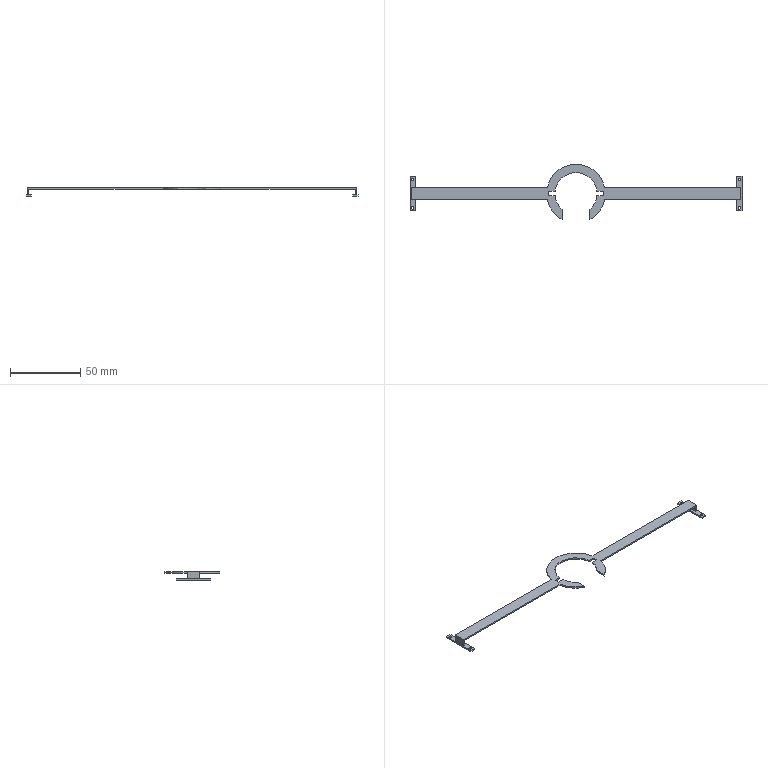Part | SolidWorks | features ICE 2, Extrusion 1 | 1 solid | 44 faces | box 236.176 x 39.297 x 6 mm | volume 2428 mm3 | plane 30 | cylinder 14 | commonest cylinder face diameters 2 x8 30 x3 41.805 x3
STEP:
#1=CARTESIAN_POINT('',(115.275,-10.,-5.));
#2=VERTEX_POINT('',#1);
#3=CARTESIAN_POINT('',(117.275,-10.,-5.));
#4=VERTEX_POINT('',#3);
#5=CARTESIAN_POINT('',(116.275,-10.,-5.));
#6=DIRECTION('',(0.,0.,1.));
#7=DIRECTION('',(-1.,0.,0.));
#8=AXIS2_PLACEMENT_3D('',#5,#6,#7);
#9=CIRCLE('',#8,1.);
#10=EDGE_CURVE('',#2,#4,#9,.T.);
#11=ORIENTED_EDGE('',*,*,#10,.T.);
#12=CARTESIAN_POINT('',(117.275,-10.,-6.));
#13=VERTEX_POINT('',#12);
#14=CARTESIAN_POINT('',(117.275,-10.,-5.));
#15=DIRECTION('',(0.,0.,-1.));
#16=VECTOR('',#15,1000.);
#17=LINE('',#14,#16);
#18=EDGE_CURVE('',#4,#13,#17,.T.);
#19=ORIENTED_EDGE('',*,*,#18,.T.);
#20=CARTESIAN_POINT('',(115.275,-10.,-6.));
#21=VERTEX_POINT('',#20);
#22=CARTESIAN_POINT('',(116.275,-10.,-6.));
#23=DIRECTION('',(0.,0.,1.));
#24=DIRECTION('',(-1.,0.,0.));
#25=AXIS2_PLACEMENT_3D('',#22,#23,#24);
#26=CIRCLE('',#25,1.);
#27=EDGE_CURVE('',#21,#13,#26,.T.);
#28=ORIENTED_EDGE('',*,*,#27,.F.);
#29=CARTESIAN_POINT('',(115.275,-10.,-5.));
#30=DIRECTION('',(0.,0.,-1.));
#31=VECTOR('',#30,1000.);
#32=LINE('',#29,#31);
#33=EDGE_CURVE('',#2,#21,#32,.T.);
#34=ORIENTED_EDGE('',*,*,#33,.F.);
#35=EDGE_LOOP('',(#11,#19,#28,#34));
#36=FACE_OUTER_BOUND('',#35,.T.);
#37=CARTESIAN_POINT('',(116.275,-10.,-5.));
#38=DIRECTION('',(0.,0.,-1.));
#39=DIRECTION('',(-1.,0.,0.));
#40=AXIS2_PLACEMENT_3D('',#37,#38,#39);
#41=CYLINDRICAL_SURFACE('',#40,1.);
#42=ADVANCED_FACE('',(#36),#41,.F.);
#43=CARTESIAN_POINT('',(115.275,10.,-5.));
#44=VERTEX_POINT('',#43);
#45=CARTESIAN_POINT('',(117.275,10.,-5.));
#46=VERTEX_POINT('',#45);
#47=CARTESIAN_POINT('',(116.275,10.,-5.));
#48=DIRECTION('',(0.,0.,1.));
#49=DIRECTION('',(-1.,0.,0.));
#50=AXIS2_PLACEMENT_3D('',#47,#48,#49);
#51=CIRCLE('',#50,1.);
#52=EDGE_CURVE('',#44,#46,#51,.T.);
#53=ORIENTED_EDGE('',*,*,#52,.T.);
#54=CARTESIAN_POINT('',(117.275,10.,-6.));
#55=VERTEX_POINT('',#54);
#56=CARTESIAN_POINT('',(117.275,10.,-5.));
#57=DIRECTION('',(0.,0.,-1.));
#58=VECTOR('',#57,1000.);
#59=LINE('',#56,#58);
#60=EDGE_CURVE('',#46,#55,#59,.T.);
#61=ORIENTED_EDGE('',*,*,#60,.T.);
#62=CARTESIAN_POINT('',(115.275,10.,-6.));
#63=VERTEX_POINT('',#62);
#64=CARTESIAN_POINT('',(116.275,10.,-6.));
#65=DIRECTION('',(0.,0.,1.));
#66=DIRECTION('',(-1.,0.,0.));
#67=AXIS2_PLACEMENT_3D('',#64,#65,#66);
#68=CIRCLE('',#67,1.);
#69=EDGE_CURVE('',#63,#55,#68,.T.);
#70=ORIENTED_EDGE('',*,*,#69,.F.);
#71=CARTESIAN_POINT('',(115.275,10.,-5.));
#72=DIRECTION('',(0.,0.,-1.));
#73=VECTOR('',#72,1000.);
#74=LINE('',#71,#73);
#75=EDGE_CURVE('',#44,#63,#74,.T.);
#76=ORIENTED_EDGE('',*,*,#75,.F.);
#77=EDGE_LOOP('',(#53,#61,#70,#76));
#78=FACE_OUTER_BOUND('',#77,.T.);
#79=CARTESIAN_POINT('',(116.275,10.,-5.));
#80=DIRECTION('',(0.,0.,-1.));
#81=DIRECTION('',(-1.,0.,0.));
#82=AXIS2_PLACEMENT_3D('',#79,#80,#81);
#83=CYLINDRICAL_SURFACE('',#82,1.);
#84=ADVANCED_FACE('',(#78),#83,.F.);
#85=CARTESIAN_POINT('',(-117.275,10.,-5.));
#86=VERTEX_POINT('',#85);
#87=CARTESIAN_POINT('',(-115.275,10.,-5.));
#88=VERTEX_POINT('',#87);
#89=CARTESIAN_POINT('',(-116.275,10.,-5.));
#90=DIRECTION('',(0.,0.,1.));
#91=DIRECTION('',(1.,0.,0.));
#92=AXIS2_PLACEMENT_3D('',#89,#90,#91);
#93=CIRCLE('',#92,1.);
#94=EDGE_CURVE('',#86,#88,#93,.T.);
#95=ORIENTED_EDGE('',*,*,#94,.T.);
#96=CARTESIAN_POINT('',(-115.275,10.,-6.));
#97=VERTEX_POINT('',#96);
#98=CARTESIAN_POINT('',(-115.275,10.,-5.));
#99=DIRECTION('',(0.,0.,-1.));
#100=VECTOR('',#99,1000.);
#101=LINE('',#98,#100);
#102=EDGE_CURVE('',#88,#97,#101,.T.);
#103=ORIENTED_EDGE('',*,*,#102,.T.);
#104=CARTESIAN_POINT('',(-117.275,10.,-6.));
#105=VERTEX_POINT('',#104);
#106=CARTESIAN_POINT('',(-116.275,10.,-6.));
#107=DIRECTION('',(0.,0.,1.));
#108=DIRECTION('',(1.,0.,0.));
#109=AXIS2_PLACEMENT_3D('',#106,#107,#108);
#110=CIRCLE('',#109,1.);
#111=EDGE_CURVE('',#105,#97,#110,.T.);
#112=ORIENTED_EDGE('',*,*,#111,.F.);
#113=CARTESIAN_POINT('',(-117.275,10.,-5.));
#114=DIRECTION('',(0.,0.,-1.));
#115=VECTOR('',#114,1000.);
#116=LINE('',#113,#115);
#117=EDGE_CURVE('',#86,#105,#116,.T.);
#118=ORIENTED_EDGE('',*,*,#117,.F.);
#119=EDGE_LOOP('',(#95,#103,#112,#118));
#120=FACE_OUTER_BOUND('',#119,.T.);
#121=CARTESIAN_POINT('',(-116.275,10.,-5.));
#122=DIRECTION('',(0.,0.,-1.));
#123=DIRECTION('',(-1.,0.,0.));
#124=AXIS2_PLACEMENT_3D('',#121,#122,#123);
#125=CYLINDRICAL_SURFACE('',#124,1.);
#126=ADVANCED_FACE('',(#120),#125,.F.);
#127=CARTESIAN_POINT('',(-117.275,-10.,-5.));
#128=VERTEX_POINT('',#127);
#129=CARTESIAN_POINT('',(-115.275,-10.,-5.));
#130=VERTEX_POINT('',#129);
#131=CARTESIAN_POINT('',(-116.275,-10.,-5.));
#132=DIRECTION('',(0.,0.,1.));
#133=DIRECTION('',(1.,0.,0.));
#134=AXIS2_PLACEMENT_3D('',#131,#132,#133);
#135=CIRCLE('',#134,1.);
#136=EDGE_CURVE('',#128,#130,#135,.T.);
#137=ORIENTED_EDGE('',*,*,#136,.T.);
#138=CARTESIAN_POINT('',(-115.275,-10.,-6.));
#139=VERTEX_POINT('',#138);
#140=CARTESIAN_POINT('',(-115.275,-10.,-5.));
#141=DIRECTION('',(0.,0.,-1.));
#142=VECTOR('',#141,1000.);
#143=LINE('',#140,#142);
#144=EDGE_CURVE('',#130,#139,#143,.T.);
#145=ORIENTED_EDGE('',*,*,#144,.T.);
#146=CARTESIAN_POINT('',(-117.275,-10.,-6.));
#147=VERTEX_POINT('',#146);
#148=CARTESIAN_POINT('',(-116.275,-10.,-6.));
#149=DIRECTION('',(0.,0.,1.));
#150=DIRECTION('',(1.,0.,0.));
#151=AXIS2_PLACEMENT_3D('',#148,#149,#150);
#152=CIRCLE('',#151,1.);
#153=EDGE_CURVE('',#147,#139,#152,.T.);
#154=ORIENTED_EDGE('',*,*,#153,.F.);
#155=CARTESIAN_POINT('',(-117.275,-10.,-5.));
#156=DIRECTION('',(0.,0.,-1.));
#157=VECTOR('',#156,1000.);
#158=LINE('',#155,#157);
#159=EDGE_CURVE('',#128,#147,#158,.T.);
#160=ORIENTED_EDGE('',*,*,#159,.F.);
#161=EDGE_LOOP('',(#137,#145,#154,#160));
#162=FACE_OUTER_BOUND('',#161,.T.);
#163=CARTESIAN_POINT('',(-116.275,-10.,-5.));
#164=DIRECTION('',(0.,0.,-1.));
#165=DIRECTION('',(-1.,0.,0.));
#166=AXIS2_PLACEMENT_3D('',#163,#164,#165);
#167=CYLINDRICAL_SURFACE('',#166,1.);
#168=ADVANCED_FACE('',(#162),#167,.F.);
#169=CARTESIAN_POINT('',(116.275,-4.349,-5.));
#170=VERTEX_POINT('',#169);
#171=CARTESIAN_POINT('',(116.275,-4.349,-1.));
#172=VERTEX_POINT('',#171);
#173=CARTESIAN_POINT('',(116.275,-4.349,-14.755));
#174=DIRECTION('',(0.,0.,1.));
#175=VECTOR('',#174,1000.);
#176=LINE('',#173,#175);
#177=EDGE_CURVE('',#170,#172,#176,.T.);
#178=ORIENTED_EDGE('',*,*,#177,.F.);
#179=CARTESIAN_POINT('',(117.275,-4.349,-5.));
#180=VERTEX_POINT('',#179);
#181=CARTESIAN_POINT('',(20.445,-4.349,-5.));
#182=DIRECTION('',(1.,0.,0.));
#183=VECTOR('',#182,1000.);
#184=LINE('',#181,#183);
#185=EDGE_CURVE('',#170,#180,#184,.T.);
#186=ORIENTED_EDGE('',*,*,#185,.T.);
#187=CARTESIAN_POINT('',(117.275,-4.349,0.));
#188=VERTEX_POINT('',#187);
#189=CARTESIAN_POINT('',(117.275,-4.349,-1.));
#190=DIRECTION('',(0.,0.,1.));
#191=VECTOR('',#190,1000.);
#192=LINE('',#189,#191);
#193=EDGE_CURVE('',#180,#188,#192,.T.);
#194=ORIENTED_EDGE('',*,*,#193,.T.);
#195=CARTESIAN_POINT('',(20.445,-4.349,0.));
#196=VERTEX_POINT('',#195);
#197=CARTESIAN_POINT('',(20.445,-4.349,0.));
#198=DIRECTION('',(1.,0.,0.));
#199=VECTOR('',#198,1000.);
#200=LINE('',#197,#199);
#201=EDGE_CURVE('',#196,#188,#200,.T.);
#202=ORIENTED_EDGE('',*,*,#201,.F.);
#203=CARTESIAN_POINT('',(20.445,-4.349,-1.));
#204=VERTEX_POINT('',#203);
#205=CARTESIAN_POINT('',(20.445,-4.349,-1.));
#206=DIRECTION('',(0.,0.,1.));
#207=VECTOR('',#206,1000.);
#208=LINE('',#205,#207);
#209=EDGE_CURVE('',#204,#196,#208,.T.);
#210=ORIENTED_EDGE('',*,*,#209,.F.);
#211=CARTESIAN_POINT('',(20.445,-4.349,-1.));
#212=DIRECTION('',(1.,0.,0.));
#213=VECTOR('',#212,1000.);
#214=LINE('',#211,#213);
#215=EDGE_CURVE('',#204,#172,#214,.T.);
#216=ORIENTED_EDGE('',*,*,#215,.T.);
#217=EDGE_LOOP('',(#178,#186,#194,#202,#210,#216));
#218=FACE_OUTER_BOUND('',#217,.T.);
#219=CARTESIAN_POINT('',(20.445,-4.349,-1.));
#220=DIRECTION('',(0.,-1.,0.));
#221=DIRECTION('',(0.,0.,-1.));
#222=AXIS2_PLACEMENT_3D('',#219,#220,#221);
#223=PLANE('',#222);
#224=ADVANCED_FACE('',(#218),#223,.T.);
#225=CARTESIAN_POINT('',(117.275,4.349,-5.));
#226=VERTEX_POINT('',#225);
#227=CARTESIAN_POINT('',(117.275,4.349,0.));
#228=VERTEX_POINT('',#227);
#229=CARTESIAN_POINT('',(117.275,4.349,-1.));
#230=DIRECTION('',(0.,0.,1.));
#231=VECTOR('',#230,1000.);
#232=LINE('',#229,#231);
#233=EDGE_CURVE('',#226,#228,#232,.T.);
#234=ORIENTED_EDGE('',*,*,#233,.F.);
#235=CARTESIAN_POINT('',(116.275,4.349,-5.));
#236=VERTEX_POINT('',#235);
#237=CARTESIAN_POINT('',(20.445,4.349,-5.));
#238=DIRECTION('',(-1.,0.,0.));
#239=VECTOR('',#238,1000.);
#240=LINE('',#237,#239);
#241=EDGE_CURVE('',#226,#236,#240,.T.);
#242=ORIENTED_EDGE('',*,*,#241,.T.);
#243=CARTESIAN_POINT('',(116.275,4.349,-1.));
#244=VERTEX_POINT('',#243);
#245=CARTESIAN_POINT('',(116.275,4.349,-14.755));
#246=DIRECTION('',(0.,0.,1.));
#247=VECTOR('',#246,1000.);
#248=LINE('',#245,#247);
#249=EDGE_CURVE('',#236,#244,#248,.T.);
#250=ORIENTED_EDGE('',*,*,#249,.T.);
#251=CARTESIAN_POINT('',(20.445,4.349,-1.));
#252=VERTEX_POINT('',#251);
#253=CARTESIAN_POINT('',(20.445,4.349,-1.));
#254=DIRECTION('',(-1.,0.,0.));
#255=VECTOR('',#254,1000.);
#256=LINE('',#253,#255);
#257=EDGE_CURVE('',#244,#252,#256,.T.);
#258=ORIENTED_EDGE('',*,*,#257,.T.);
#259=CARTESIAN_POINT('',(20.445,4.349,0.));
#260=VERTEX_POINT('',#259);
#261=CARTESIAN_POINT('',(20.445,4.349,-1.));
#262=DIRECTION('',(0.,0.,1.));
#263=VECTOR('',#262,1000.);
#264=LINE('',#261,#263);
#265=EDGE_CURVE('',#252,#260,#264,.T.);
#266=ORIENTED_EDGE('',*,*,#265,.T.);
#267=CARTESIAN_POINT('',(20.445,4.349,0.));
#268=DIRECTION('',(-1.,0.,0.));
#269=VECTOR('',#268,1000.);
#270=LINE('',#267,#269);
#271=EDGE_CURVE('',#228,#260,#270,.T.);
#272=ORIENTED_EDGE('',*,*,#271,.F.);
#273=EDGE_LOOP('',(#234,#242,#250,#258,#266,#272));
#274=FACE_OUTER_BOUND('',#273,.T.);
#275=CARTESIAN_POINT('',(20.445,4.349,-1.));
#276=DIRECTION('',(0.,1.,0.));
#277=DIRECTION('',(0.,0.,1.));
#278=AXIS2_PLACEMENT_3D('',#275,#276,#277);
#279=PLANE('',#278);
#280=ADVANCED_FACE('',(#274),#279,.T.);
#281=ORIENTED_EDGE('',*,*,#193,.F.);
#282=CARTESIAN_POINT('',(117.275,4.349,-5.));
#283=DIRECTION('',(0.,1.,0.));
#284=VECTOR('',#283,1000.);
#285=LINE('',#282,#284);
#286=EDGE_CURVE('',#180,#226,#285,.T.);
#287=ORIENTED_EDGE('',*,*,#286,.T.);
#288=ORIENTED_EDGE('',*,*,#233,.T.);
#289=CARTESIAN_POINT('',(117.275,4.349,0.));
#290=DIRECTION('',(0.,1.,0.));
#291=VECTOR('',#290,1000.);
#292=LINE('',#289,#291);
#293=EDGE_CURVE('',#188,#228,#292,.T.);
#294=ORIENTED_EDGE('',*,*,#293,.F.);
#295=EDGE_LOOP('',(#281,#287,#288,#294));
#296=FACE_OUTER_BOUND('',#295,.T.);
#297=CARTESIAN_POINT('',(117.275,4.349,-1.));
#298=DIRECTION('',(1.,0.,0.));
#299=DIRECTION('',(0.,0.,-1.));
#300=AXIS2_PLACEMENT_3D('',#297,#298,#299);
#301=PLANE('',#300);
#302=ADVANCED_FACE('',(#296),#301,.T.);
#303=ORIENTED_EDGE('',*,*,#249,.F.);
#304=CARTESIAN_POINT('',(116.275,4.349,-5.));
#305=DIRECTION('',(0.,-1.,0.));
#306=VECTOR('',#305,1000.);
#307=LINE('',#304,#306);
#308=EDGE_CURVE('',#236,#170,#307,.T.);
#309=ORIENTED_EDGE('',*,*,#308,.T.);
#310=ORIENTED_EDGE('',*,*,#177,.T.);
#311=CARTESIAN_POINT('',(116.275,0.,-1.));
#312=DIRECTION('',(0.,-1.,0.));
#313=VECTOR('',#312,1000.);
#314=LINE('',#311,#313);
#315=EDGE_CURVE('',#244,#172,#314,.T.);
#316=ORIENTED_EDGE('',*,*,#315,.F.);
#317=EDGE_LOOP('',(#303,#309,#310,#316));
#318=FACE_OUTER_BOUND('',#317,.T.);
#319=CARTESIAN_POINT('',(116.275,4.349,-14.755));
#320=DIRECTION('',(-1.,0.,0.));
#321=DIRECTION('',(0.,0.,1.));
#322=AXIS2_PLACEMENT_3D('',#319,#320,#321);
#323=PLANE('',#322);
#324=ADVANCED_FACE('',(#318),#323,.T.);
#325=CARTESIAN_POINT('',(9.927,-18.395,0.));
#326=VERTEX_POINT('',#325);
#327=CARTESIAN_POINT('',(0.,0.,0.));
#328=DIRECTION('',(0.,0.,1.));
#329=DIRECTION('',(1.,0.,0.));
#330=AXIS2_PLACEMENT_3D('',#327,#328,#329);
#331=CIRCLE('',#330,20.903);
#332=EDGE_CURVE('',#326,#196,#331,.T.);
#333=ORIENTED_EDGE('',*,*,#332,.F.);
#334=CARTESIAN_POINT('',(9.927,-18.395,-1.));
#335=VERTEX_POINT('',#334);
#336=CARTESIAN_POINT('',(9.927,-18.395,-1.));
#337=DIRECTION('',(0.,0.,1.));
#338=VECTOR('',#337,1000.);
#339=LINE('',#336,#338);
#340=EDGE_CURVE('',#335,#326,#339,.T.);
#341=ORIENTED_EDGE('',*,*,#340,.F.);
#342=CARTESIAN_POINT('',(0.,0.,-1.));
#343=DIRECTION('',(0.,0.,1.));
#344=DIRECTION('',(1.,0.,0.));
#345=AXIS2_PLACEMENT_3D('',#342,#343,#344);
#346=CIRCLE('',#345,20.903);
#347=EDGE_CURVE('',#335,#204,#346,.T.);
#348=ORIENTED_EDGE('',*,*,#347,.T.);
#349=ORIENTED_EDGE('',*,*,#209,.T.);
#350=EDGE_LOOP('',(#333,#341,#348,#349));
#351=FACE_OUTER_BOUND('',#350,.T.);
#352=CARTESIAN_POINT('',(0.,0.,-1.));
#353=DIRECTION('',(0.,0.,1.));
#354=DIRECTION('',(1.,0.,0.));
#355=AXIS2_PLACEMENT_3D('',#352,#353,#354);
#356=CYLINDRICAL_SURFACE('',#355,20.903);
#357=ADVANCED_FACE('',(#351),#356,.T.);
#358=CARTESIAN_POINT('',(9.927,-11.245,0.));
#359=VERTEX_POINT('',#358);
#360=CARTESIAN_POINT('',(9.927,-11.245,0.));
#361=DIRECTION('',(0.,-1.,0.));
#362=VECTOR('',#361,1000.);
#363=LINE('',#360,#362);
#364=EDGE_CURVE('',#359,#326,#363,.T.);
#365=ORIENTED_EDGE('',*,*,#364,.F.);
#366=CARTESIAN_POINT('',(9.927,-11.245,-1.));
#367=VERTEX_POINT('',#366);
#368=CARTESIAN_POINT('',(9.927,-11.245,-1.));
#369=DIRECTION('',(0.,0.,1.));
#370=VECTOR('',#369,1000.);
#371=LINE('',#368,#370);
#372=EDGE_CURVE('',#367,#359,#371,.T.);
#373=ORIENTED_EDGE('',*,*,#372,.F.);
#374=CARTESIAN_POINT('',(9.927,-11.245,-1.));
#375=DIRECTION('',(0.,-1.,0.));
#376=VECTOR('',#375,1000.);
#377=LINE('',#374,#376);
#378=EDGE_CURVE('',#367,#335,#377,.T.);
#379=ORIENTED_EDGE('',*,*,#378,.T.);
#380=ORIENTED_EDGE('',*,*,#340,.T.);
#381=EDGE_LOOP('',(#365,#373,#379,#380));
#382=FACE_OUTER_BOUND('',#381,.T.);
#383=CARTESIAN_POINT('',(9.927,-11.245,-1.));
#384=DIRECTION('',(-1.,0.,0.));
#385=DIRECTION('',(0.,0.,1.));
#386=AXIS2_PLACEMENT_3D('',#383,#384,#385);
#387=PLANE('',#386);
#388=ADVANCED_FACE('',(#382),#387,.T.);
#389=CARTESIAN_POINT('',(14.91,-1.641,0.));
#390=VERTEX_POINT('',#389);
#391=CARTESIAN_POINT('',(0.,0.,0.));
#392=DIRECTION('',(0.,0.,-1.));
#393=DIRECTION('',(1.,0.,0.));
#394=AXIS2_PLACEMENT_3D('',#391,#392,#393);
#395=CIRCLE('',#394,15.);
#396=EDGE_CURVE('',#390,#359,#395,.T.);
#397=ORIENTED_EDGE('',*,*,#396,.F.);
#398=CARTESIAN_POINT('',(14.91,-1.641,-1.));
#399=VERTEX_POINT('',#398);
#400=CARTESIAN_POINT('',(14.91,-1.641,-1.));
#401=DIRECTION('',(0.,0.,1.));
#402=VECTOR('',#401,1000.);
#403=LINE('',#400,#402);
#404=EDGE_CURVE('',#399,#390,#403,.T.);
#405=ORIENTED_EDGE('',*,*,#404,.F.);
#406=CARTESIAN_POINT('',(0.,0.,-1.));
#407=DIRECTION('',(0.,0.,-1.));
#408=DIRECTION('',(1.,0.,0.));
#409=AXIS2_PLACEMENT_3D('',#406,#407,#408);
#410=CIRCLE('',#409,15.);
#411=EDGE_CURVE('',#399,#367,#410,.T.);
#412=ORIENTED_EDGE('',*,*,#411,.T.);
#413=ORIENTED_EDGE('',*,*,#372,.T.);
#414=EDGE_LOOP('',(#397,#405,#412,#413));
#415=FACE_OUTER_BOUND('',#414,.T.);
#416=CARTESIAN_POINT('',(0.,0.,-1.));
#417=DIRECTION('',(0.,0.,1.));
#418=DIRECTION('',(1.,0.,0.));
#419=AXIS2_PLACEMENT_3D('',#416,#417,#418);
#420=CYLINDRICAL_SURFACE('',#419,15.);
#421=ADVANCED_FACE('',(#415),#420,.F.);
#422=CARTESIAN_POINT('',(19.244,-1.641,0.));
#423=VERTEX_POINT('',#422);
#424=CARTESIAN_POINT('',(14.91,-1.641,0.));
#425=DIRECTION('',(-1.,0.,0.));
#426=VECTOR('',#425,1000.);
#427=LINE('',#424,#426);
#428=EDGE_CURVE('',#423,#390,#427,.T.);
#429=ORIENTED_EDGE('',*,*,#428,.F.);
#430=CARTESIAN_POINT('',(19.244,-1.641,-1.));
#431=VERTEX_POINT('',#430);
#432=CARTESIAN_POINT('',(19.244,-1.641,-1.));
#433=DIRECTION('',(0.,0.,1.));
#434=VECTOR('',#433,1000.);
#435=LINE('',#432,#434);
#436=EDGE_CURVE('',#431,#423,#435,.T.);
#437=ORIENTED_EDGE('',*,*,#436,.F.);
#438=CARTESIAN_POINT('',(14.91,-1.641,-1.));
#439=DIRECTION('',(-1.,0.,0.));
#440=VECTOR('',#439,1000.);
#441=LINE('',#438,#440);
#442=EDGE_CURVE('',#431,#399,#441,.T.);
#443=ORIENTED_EDGE('',*,*,#442,.T.);
#444=ORIENTED_EDGE('',*,*,#404,.T.);
#445=EDGE_LOOP('',(#429,#437,#443,#444));
#446=FACE_OUTER_BOUND('',#445,.T.);
#447=CARTESIAN_POINT('',(14.91,-1.641,-1.));
#448=DIRECTION('',(0.,1.,0.));
#449=DIRECTION('',(0.,0.,1.));
#450=AXIS2_PLACEMENT_3D('',#447,#448,#449);
#451=PLANE('',#450);
#452=ADVANCED_FACE('',(#446),#451,.T.);
#453=CARTESIAN_POINT('',(19.244,1.641,0.));
#454=VERTEX_POINT('',#453);
#455=CARTESIAN_POINT('',(19.244,-1.641,0.));
#456=DIRECTION('',(0.,-1.,0.));
#457=VECTOR('',#456,1000.);
#458=LINE('',#455,#457);
#459=EDGE_CURVE('',#454,#423,#458,.T.);
#460=ORIENTED_EDGE('',*,*,#459,.F.);
#461=CARTESIAN_POINT('',(19.244,1.641,-1.));
#462=VERTEX_POINT('',#461);
#463=CARTESIAN_POINT('',(19.244,1.641,-1.));
#464=DIRECTION('',(0.,0.,1.));
#465=VECTOR('',#464,1000.);
#466=LINE('',#463,#465);
#467=EDGE_CURVE('',#462,#454,#466,.T.);
#468=ORIENTED_EDGE('',*,*,#467,.F.);
#469=CARTESIAN_POINT('',(19.244,-1.641,-1.));
#470=DIRECTION('',(0.,-1.,0.));
#471=VECTOR('',#470,1000.);
#472=LINE('',#469,#471);
#473=EDGE_CURVE('',#462,#431,#472,.T.);
#474=ORIENTED_EDGE('',*,*,#473,.T.);
#475=ORIENTED_EDGE('',*,*,#436,.T.);
#476=EDGE_LOOP('',(#460,#468,#474,#475));
#477=FACE_OUTER_BOUND('',#476,.T.);
#478=CARTESIAN_POINT('',(19.244,-1.641,-1.));
#479=DIRECTION('',(-1.,0.,0.));
#480=DIRECTION('',(0.,0.,1.));
#481=AXIS2_PLACEMENT_3D('',#478,#479,#480);
#482=PLANE('',#481);
#483=ADVANCED_FACE('',(#477),#482,.T.);
#484=CARTESIAN_POINT('',(14.91,1.641,0.));
#485=VERTEX_POINT('',#484);
#486=CARTESIAN_POINT('',(14.91,1.641,0.));
#487=DIRECTION('',(1.,0.,0.));
#488=VECTOR('',#487,1000.);
#489=LINE('',#486,#488);
#490=EDGE_CURVE('',#485,#454,#489,.T.);
#491=ORIENTED_EDGE('',*,*,#490,.F.);
#492=CARTESIAN_POINT('',(14.91,1.641,-1.));
#493=VERTEX_POINT('',#492);
#494=CARTESIAN_POINT('',(14.91,1.641,-1.));
#495=DIRECTION('',(0.,0.,1.));
#496=VECTOR('',#495,1000.);
#497=LINE('',#494,#496);
#498=EDGE_CURVE('',#493,#485,#497,.T.);
#499=ORIENTED_EDGE('',*,*,#498,.F.);
#500=CARTESIAN_POINT('',(14.91,1.641,-1.));
#501=DIRECTION('',(1.,0.,0.));
#502=VECTOR('',#501,1000.);
#503=LINE('',#500,#502);
#504=EDGE_CURVE('',#493,#462,#503,.T.);
#505=ORIENTED_EDGE('',*,*,#504,.T.);
#506=ORIENTED_EDGE('',*,*,#467,.T.);
#507=EDGE_LOOP('',(#491,#499,#505,#506));
#508=FACE_OUTER_BOUND('',#507,.T.);
#509=CARTESIAN_POINT('',(14.91,1.641,-1.));
#510=DIRECTION('',(0.,-1.,0.));
#511=DIRECTION('',(0.,0.,-1.));
#512=AXIS2_PLACEMENT_3D('',#509,#510,#511);
#513=PLANE('',#512);
#514=ADVANCED_FACE('',(#508),#513,.T.);
#515=CARTESIAN_POINT('',(-14.91,1.641,0.));
#516=VERTEX_POINT('',#515);
#517=CARTESIAN_POINT('',(0.,0.,0.));
#518=DIRECTION('',(0.,0.,-1.));
#519=DIRECTION('',(1.,0.,0.));
#520=AXIS2_PLACEMENT_3D('',#517,#518,#519);
#521=CIRCLE('',#520,15.);
#522=EDGE_CURVE('',#516,#485,#521,.T.);
#523=ORIENTED_EDGE('',*,*,#522,.F.);
#524=CARTESIAN_POINT('',(-14.91,1.641,-1.));
#525=VERTEX_POINT('',#524);
#526=CARTESIAN_POINT('',(-14.91,1.641,-1.));
#527=DIRECTION('',(0.,0.,1.));
#528=VECTOR('',#527,1000.);
#529=LINE('',#526,#528);
#530=EDGE_CURVE('',#525,#516,#529,.T.);
#531=ORIENTED_EDGE('',*,*,#530,.F.);
#532=CARTESIAN_POINT('',(0.,0.,-1.));
#533=DIRECTION('',(0.,0.,-1.));
#534=DIRECTION('',(1.,0.,0.));
#535=AXIS2_PLACEMENT_3D('',#532,#533,#534);
#536=CIRCLE('',#535,15.);
#537=EDGE_CURVE('',#525,#493,#536,.T.);
#538=ORIENTED_EDGE('',*,*,#537,.T.);
#539=ORIENTED_EDGE('',*,*,#498,.T.);
#540=EDGE_LOOP('',(#523,#531,#538,#539));
#541=FACE_OUTER_BOUND('',#540,.T.);
#542=CARTESIAN_POINT('',(0.,0.,-1.));
#543=DIRECTION('',(0.,0.,1.));
#544=DIRECTION('',(1.,0.,0.));
#545=AXIS2_PLACEMENT_3D('',#542,#543,#544);
#546=CYLINDRICAL_SURFACE('',#545,15.);
#547=ADVANCED_FACE('',(#541),#546,.F.);
#548=CARTESIAN_POINT('',(-19.244,1.641,0.));
#549=VERTEX_POINT('',#548);
#550=CARTESIAN_POINT('',(-19.244,1.641,0.));
#551=DIRECTION('',(1.,0.,0.));
#552=VECTOR('',#551,1000.);
#553=LINE('',#550,#552);
#554=EDGE_CURVE('',#549,#516,#553,.T.);
#555=ORIENTED_EDGE('',*,*,#554,.F.);
#556=CARTESIAN_POINT('',(-19.244,1.641,-1.));
#557=VERTEX_POINT('',#556);
#558=CARTESIAN_POINT('',(-19.244,1.641,-1.));
#559=DIRECTION('',(0.,0.,1.));
#560=VECTOR('',#559,1000.);
#561=LINE('',#558,#560);
#562=EDGE_CURVE('',#557,#549,#561,.T.);
#563=ORIENTED_EDGE('',*,*,#562,.F.);
#564=CARTESIAN_POINT('',(-19.244,1.641,-1.));
#565=DIRECTION('',(1.,0.,0.));
#566=VECTOR('',#565,1000.);
#567=LINE('',#564,#566);
#568=EDGE_CURVE('',#557,#525,#567,.T.);
#569=ORIENTED_EDGE('',*,*,#568,.T.);
#570=ORIENTED_EDGE('',*,*,#530,.T.);
#571=EDGE_LOOP('',(#555,#563,#569,#570));
#572=FACE_OUTER_BOUND('',#571,.T.);
#573=CARTESIAN_POINT('',(-19.244,1.641,-1.));
#574=DIRECTION('',(0.,-1.,0.));
#575=DIRECTION('',(0.,0.,-1.));
#576=AXIS2_PLACEMENT_3D('',#573,#574,#575);
#577=PLANE('',#576);
#578=ADVANCED_FACE('',(#572),#577,.T.);
#579=CARTESIAN_POINT('',(-19.244,-1.641,0.));
#580=VERTEX_POINT('',#579);
#581=CARTESIAN_POINT('',(-19.244,-1.641,0.));
#582=DIRECTION('',(0.,1.,0.));
#583=VECTOR('',#582,1000.);
#584=LINE('',#581,#583);
#585=EDGE_CURVE('',#580,#549,#584,.T.);
#586=ORIENTED_EDGE('',*,*,#585,.F.);
#587=CARTESIAN_POINT('',(-19.244,-1.641,-1.));
#588=VERTEX_POINT('',#587);
#589=CARTESIAN_POINT('',(-19.244,-1.641,-1.));
#590=DIRECTION('',(0.,0.,1.));
#591=VECTOR('',#590,1000.);
#592=LINE('',#589,#591);
#593=EDGE_CURVE('',#588,#580,#592,.T.);
#594=ORIENTED_EDGE('',*,*,#593,.F.);
#595=CARTESIAN_POINT('',(-19.244,-1.641,-1.));
#596=DIRECTION('',(0.,1.,0.));
#597=VECTOR('',#596,1000.);
#598=LINE('',#595,#597);
#599=EDGE_CURVE('',#588,#557,#598,.T.);
#600=ORIENTED_EDGE('',*,*,#599,.T.);
#601=ORIENTED_EDGE('',*,*,#562,.T.);
#602=EDGE_LOOP('',(#586,#594,#600,#601));
#603=FACE_OUTER_BOUND('',#602,.T.);
#604=CARTESIAN_POINT('',(-19.244,-1.641,-1.));
#605=DIRECTION('',(1.,0.,0.));
#606=DIRECTION('',(0.,0.,-1.));
#607=AXIS2_PLACEMENT_3D('',#604,#605,#606);
#608=PLANE('',#607);
#609=ADVANCED_FACE('',(#603),#608,.T.);
#610=CARTESIAN_POINT('',(-14.91,-1.641,0.));
#611=VERTEX_POINT('',#610);
#612=CARTESIAN_POINT('',(-19.244,-1.641,0.));
#613=DIRECTION('',(-1.,0.,0.));
#614=VECTOR('',#613,1000.);
#615=LINE('',#612,#614);
#616=EDGE_CURVE('',#611,#580,#615,.T.);
#617=ORIENTED_EDGE('',*,*,#616,.F.);
#618=CARTESIAN_POINT('',(-14.91,-1.641,-1.));
#619=VERTEX_POINT('',#618);
#620=CARTESIAN_POINT('',(-14.91,-1.641,-1.));
#621=DIRECTION('',(0.,0.,1.));
#622=VECTOR('',#621,1000.);
#623=LINE('',#620,#622);
#624=EDGE_CURVE('',#619,#611,#623,.T.);
#625=ORIENTED_EDGE('',*,*,#624,.F.);
#626=CARTESIAN_POINT('',(-19.244,-1.641,-1.));
#627=DIRECTION('',(-1.,0.,0.));
#628=VECTOR('',#627,1000.);
#629=LINE('',#626,#628);
#630=EDGE_CURVE('',#619,#588,#629,.T.);
#631=ORIENTED_EDGE('',*,*,#630,.T.);
#632=ORIENTED_EDGE('',*,*,#593,.T.);
#633=EDGE_LOOP('',(#617,#625,#631,#632));
#634=FACE_OUTER_BOUND('',#633,.T.);
#635=CARTESIAN_POINT('',(-19.244,-1.641,-1.));
#636=DIRECTION('',(0.,1.,0.));
#637=DIRECTION('',(0.,0.,1.));
#638=AXIS2_PLACEMENT_3D('',#635,#636,#637);
#639=PLANE('',#638);
#640=ADVANCED_FACE('',(#634),#639,.T.);
#641=CARTESIAN_POINT('',(-9.927,-11.245,0.));
#642=VERTEX_POINT('',#641);
#643=CARTESIAN_POINT('',(0.,0.,0.));
#644=DIRECTION('',(0.,0.,-1.));
#645=DIRECTION('',(1.,0.,0.));
#646=AXIS2_PLACEMENT_3D('',#643,#644,#645);
#647=CIRCLE('',#646,15.);
#648=EDGE_CURVE('',#642,#611,#647,.T.);
#649=ORIENTED_EDGE('',*,*,#648,.F.);
#650=CARTESIAN_POINT('',(-9.927,-11.245,-1.));
#651=VERTEX_POINT('',#650);
#652=CARTESIAN_POINT('',(-9.927,-11.245,-1.));
#653=DIRECTION('',(0.,0.,1.));
#654=VECTOR('',#653,1000.);
#655=LINE('',#652,#654);
#656=EDGE_CURVE('',#651,#642,#655,.T.);
#657=ORIENTED_EDGE('',*,*,#656,.F.);
#658=CARTESIAN_POINT('',(0.,0.,-1.));
#659=DIRECTION('',(0.,0.,-1.));
#660=DIRECTION('',(1.,0.,0.));
#661=AXIS2_PLACEMENT_3D('',#658,#659,#660);
#662=CIRCLE('',#661,15.);
#663=EDGE_CURVE('',#651,#619,#662,.T.);
#664=ORIENTED_EDGE('',*,*,#663,.T.);
#665=ORIENTED_EDGE('',*,*,#624,.T.);
#666=EDGE_LOOP('',(#649,#657,#664,#665));
#667=FACE_OUTER_BOUND('',#666,.T.);
#668=CARTESIAN_POINT('',(0.,0.,-1.));
#669=DIRECTION('',(0.,0.,1.));
#670=DIRECTION('',(1.,0.,0.));
#671=AXIS2_PLACEMENT_3D('',#668,#669,#670);
#672=CYLINDRICAL_SURFACE('',#671,15.);
#673=ADVANCED_FACE('',(#667),#672,.F.);
#674=CARTESIAN_POINT('',(-9.927,-18.395,0.));
#675=VERTEX_POINT('',#674);
#676=CARTESIAN_POINT('',(-9.927,-11.245,0.));
#677=DIRECTION('',(0.,1.,0.));
#678=VECTOR('',#677,1000.);
#679=LINE('',#676,#678);
#680=EDGE_CURVE('',#675,#642,#679,.T.);
#681=ORIENTED_EDGE('',*,*,#680,.F.);
#682=CARTESIAN_POINT('',(-9.927,-18.395,-1.));
#683=VERTEX_POINT('',#682);
#684=CARTESIAN_POINT('',(-9.927,-18.395,-1.));
#685=DIRECTION('',(0.,0.,1.));
#686=VECTOR('',#685,1000.);
#687=LINE('',#684,#686);
#688=EDGE_CURVE('',#683,#675,#687,.T.);
#689=ORIENTED_EDGE('',*,*,#688,.F.);
#690=CARTESIAN_POINT('',(-9.927,-11.245,-1.));
#691=DIRECTION('',(0.,1.,0.));
#692=VECTOR('',#691,1000.);
#693=LINE('',#690,#692);
#694=EDGE_CURVE('',#683,#651,#693,.T.);
#695=ORIENTED_EDGE('',*,*,#694,.T.);
#696=ORIENTED_EDGE('',*,*,#656,.T.);
#697=EDGE_LOOP('',(#681,#689,#695,#696));
#698=FACE_OUTER_BOUND('',#697,.T.);
#699=CARTESIAN_POINT('',(-9.927,-11.245,-1.));
#700=DIRECTION('',(1.,0.,0.));
#701=DIRECTION('',(0.,0.,-1.));
#702=AXIS2_PLACEMENT_3D('',#699,#700,#701);
#703=PLANE('',#702);
#704=ADVANCED_FACE('',(#698),#703,.T.);
#705=CARTESIAN_POINT('',(-20.445,-4.349,0.));
#706=VERTEX_POINT('',#705);
#707=CARTESIAN_POINT('',(0.,0.,0.));
#708=DIRECTION('',(0.,0.,1.));
#709=DIRECTION('',(1.,0.,0.));
#710=AXIS2_PLACEMENT_3D('',#707,#708,#709);
#711=CIRCLE('',#710,20.903);
#712=EDGE_CURVE('',#706,#675,#711,.T.);
#713=ORIENTED_EDGE('',*,*,#712,.F.);
#714=CARTESIAN_POINT('',(-20.445,-4.349,-1.));
#715=VERTEX_POINT('',#714);
#716=CARTESIAN_POINT('',(-20.445,-4.349,-1.));
#717=DIRECTION('',(0.,0.,1.));
#718=VECTOR('',#717,1000.);
#719=LINE('',#716,#718);
#720=EDGE_CURVE('',#715,#706,#719,.T.);
#721=ORIENTED_EDGE('',*,*,#720,.F.);
#722=CARTESIAN_POINT('',(0.,0.,-1.));
#723=DIRECTION('',(0.,0.,1.));
#724=DIRECTION('',(1.,0.,0.));
#725=AXIS2_PLACEMENT_3D('',#722,#723,#724);
#726=CIRCLE('',#725,20.903);
#727=EDGE_CURVE('',#715,#683,#726,.T.);
#728=ORIENTED_EDGE('',*,*,#727,.T.);
#729=ORIENTED_EDGE('',*,*,#688,.T.);
#730=EDGE_LOOP('',(#713,#721,#728,#729));
#731=FACE_OUTER_BOUND('',#730,.T.);
#732=CARTESIAN_POINT('',(0.,0.,-1.));
#733=DIRECTION('',(0.,0.,1.));
#734=DIRECTION('',(1.,0.,0.));
#735=AXIS2_PLACEMENT_3D('',#732,#733,#734);
#736=CYLINDRICAL_SURFACE('',#735,20.903);
#737=ADVANCED_FACE('',(#731),#736,.T.);
#738=CARTESIAN_POINT('',(-116.275,-4.349,-5.));
#739=VERTEX_POINT('',#738);
#740=CARTESIAN_POINT('',(-117.275,-4.349,-5.));
#741=VERTEX_POINT('',#740);
#742=CARTESIAN_POINT('',(-117.275,-4.349,-5.));
#743=DIRECTION('',(-1.,0.,0.));
#744=VECTOR('',#743,1000.);
#745=LINE('',#742,#744);
#746=EDGE_CURVE('',#739,#741,#745,.T.);
#747=ORIENTED_EDGE('',*,*,#746,.F.);
#748=CARTESIAN_POINT('',(-116.275,-4.349,-1.));
#749=VERTEX_POINT('',#748);
#750=CARTESIAN_POINT('',(-116.275,-4.349,-14.755));
#751=DIRECTION('',(0.,0.,1.));
#752=VECTOR('',#751,1000.);
#753=LINE('',#750,#752);
#754=EDGE_CURVE('',#739,#749,#753,.T.);
#755=ORIENTED_EDGE('',*,*,#754,.T.);
#756=CARTESIAN_POINT('',(-117.275,-4.349,-1.));
#757=DIRECTION('',(1.,0.,0.));
#758=VECTOR('',#757,1000.);
#759=LINE('',#756,#758);
#760=EDGE_CURVE('',#749,#715,#759,.T.);
#761=ORIENTED_EDGE('',*,*,#760,.T.);
#762=ORIENTED_EDGE('',*,*,#720,.T.);
#763=CARTESIAN_POINT('',(-117.275,-4.349,0.));
#764=VERTEX_POINT('',#763);
#765=CARTESIAN_POINT('',(-117.275,-4.349,0.));
#766=DIRECTION('',(1.,0.,0.));
#767=VECTOR('',#766,1000.);
#768=LINE('',#765,#767);
#769=EDGE_CURVE('',#764,#706,#768,.T.);
#770=ORIENTED_EDGE('',*,*,#769,.F.);
#771=CARTESIAN_POINT('',(-117.275,-4.349,-1.));
#772=DIRECTION('',(0.,0.,1.));
#773=VECTOR('',#772,1000.);
#774=LINE('',#771,#773);
#775=EDGE_CURVE('',#741,#764,#774,.T.);
#776=ORIENTED_EDGE('',*,*,#775,.F.);
#777=EDGE_LOOP('',(#747,#755,#761,#762,#770,#776));
#778=FACE_OUTER_BOUND('',#777,.T.);
#779=CARTESIAN_POINT('',(-117.275,-4.349,-1.));
#780=DIRECTION('',(0.,-1.,0.));
#781=DIRECTION('',(0.,0.,-1.));
#782=AXIS2_PLACEMENT_3D('',#779,#780,#781);
#783=PLANE('',#782);
#784=ADVANCED_FACE('',(#778),#783,.T.);
#785=CARTESIAN_POINT('',(-117.275,4.349,-5.));
#786=VERTEX_POINT('',#785);
#787=CARTESIAN_POINT('',(-117.275,4.349,-5.));
#788=DIRECTION('',(0.,1.,0.));
#789=VECTOR('',#788,1000.);
#790=LINE('',#787,#789);
#791=EDGE_CURVE('',#741,#786,#790,.T.);
#792=ORIENTED_EDGE('',*,*,#791,.F.);
#793=ORIENTED_EDGE('',*,*,#775,.T.);
#794=CARTESIAN_POINT('',(-117.275,4.349,0.));
#795=VERTEX_POINT('',#794);
#796=CARTESIAN_POINT('',(-117.275,4.349,0.));
#797=DIRECTION('',(0.,-1.,0.));
#798=VECTOR('',#797,1000.);
#799=LINE('',#796,#798);
#800=EDGE_CURVE('',#795,#764,#799,.T.);
#801=ORIENTED_EDGE('',*,*,#800,.F.);
#802=CARTESIAN_POINT('',(-117.275,4.349,-1.));
#803=DIRECTION('',(0.,0.,1.));
#804=VECTOR('',#803,1000.);
#805=LINE('',#802,#804);
#806=EDGE_CURVE('',#786,#795,#805,.T.);
#807=ORIENTED_EDGE('',*,*,#806,.F.);
#808=EDGE_LOOP('',(#792,#793,#801,#807));
#809=FACE_OUTER_BOUND('',#808,.T.);
#810=CARTESIAN_POINT('',(-117.275,4.349,-1.));
#811=DIRECTION('',(-1.,0.,0.));
#812=DIRECTION('',(0.,0.,1.));
#813=AXIS2_PLACEMENT_3D('',#810,#811,#812);
#814=PLANE('',#813);
#815=ADVANCED_FACE('',(#809),#814,.T.);
#816=CARTESIAN_POINT('',(-116.275,4.349,-5.));
#817=VERTEX_POINT('',#816);
#818=CARTESIAN_POINT('',(-117.275,4.349,-5.));
#819=DIRECTION('',(1.,0.,0.));
#820=VECTOR('',#819,1000.);
#821=LINE('',#818,#820);
#822=EDGE_CURVE('',#786,#817,#821,.T.);
#823=ORIENTED_EDGE('',*,*,#822,.F.);
#824=ORIENTED_EDGE('',*,*,#806,.T.);
#825=CARTESIAN_POINT('',(-20.445,4.349,0.));
#826=VERTEX_POINT('',#825);
#827=CARTESIAN_POINT('',(-117.275,4.349,0.));
#828=DIRECTION('',(-1.,0.,0.));
#829=VECTOR('',#828,1000.);
#830=LINE('',#827,#829);
#831=EDGE_CURVE('',#826,#795,#830,.T.);
#832=ORIENTED_EDGE('',*,*,#831,.F.);
#833=CARTESIAN_POINT('',(-20.445,4.349,-1.));
#834=VERTEX_POINT('',#833);
#835=CARTESIAN_POINT('',(-20.445,4.349,-1.));
#836=DIRECTION('',(0.,0.,1.));
#837=VECTOR('',#836,1000.);
#838=LINE('',#835,#837);
#839=EDGE_CURVE('',#834,#826,#838,.T.);
#840=ORIENTED_EDGE('',*,*,#839,.F.);
#841=CARTESIAN_POINT('',(-116.275,4.349,-1.));
#842=VERTEX_POINT('',#841);
#843=CARTESIAN_POINT('',(-117.275,4.349,-1.));
#844=DIRECTION('',(-1.,0.,0.));
#845=VECTOR('',#844,1000.);
#846=LINE('',#843,#845);
#847=EDGE_CURVE('',#834,#842,#846,.T.);
#848=ORIENTED_EDGE('',*,*,#847,.T.);
#849=CARTESIAN_POINT('',(-116.275,4.349,-14.755));
#850=DIRECTION('',(0.,0.,1.));
#851=VECTOR('',#850,1000.);
#852=LINE('',#849,#851);
#853=EDGE_CURVE('',#817,#842,#852,.T.);
#854=ORIENTED_EDGE('',*,*,#853,.F.);
#855=EDGE_LOOP('',(#823,#824,#832,#840,#848,#854));
#856=FACE_OUTER_BOUND('',#855,.T.);
#857=CARTESIAN_POINT('',(-117.275,4.349,-1.));
#858=DIRECTION('',(0.,1.,0.));
#859=DIRECTION('',(0.,0.,1.));
#860=AXIS2_PLACEMENT_3D('',#857,#858,#859);
#861=PLANE('',#860);
#862=ADVANCED_FACE('',(#856),#861,.T.);
#863=CARTESIAN_POINT('',(0.,0.,0.));
#864=DIRECTION('',(0.,0.,1.));
#865=DIRECTION('',(1.,0.,0.));
#866=AXIS2_PLACEMENT_3D('',#863,#864,#865);
#867=CIRCLE('',#866,20.903);
#868=EDGE_CURVE('',#260,#826,#867,.T.);
#869=ORIENTED_EDGE('',*,*,#868,.F.);
#870=ORIENTED_EDGE('',*,*,#265,.F.);
#871=CARTESIAN_POINT('',(0.,0.,-1.));
#872=DIRECTION('',(0.,0.,1.));
#873=DIRECTION('',(1.,0.,0.));
#874=AXIS2_PLACEMENT_3D('',#871,#872,#873);
#875=CIRCLE('',#874,20.903);
#876=EDGE_CURVE('',#252,#834,#875,.T.);
#877=ORIENTED_EDGE('',*,*,#876,.T.);
#878=ORIENTED_EDGE('',*,*,#839,.T.);
#879=EDGE_LOOP('',(#869,#870,#877,#878));
#880=FACE_OUTER_BOUND('',#879,.T.);
#881=CARTESIAN_POINT('',(0.,0.,-1.));
#882=DIRECTION('',(0.,0.,1.));
#883=DIRECTION('',(1.,0.,0.));
#884=AXIS2_PLACEMENT_3D('',#881,#882,#883);
#885=CYLINDRICAL_SURFACE('',#884,20.903);
#886=ADVANCED_FACE('',(#880),#885,.T.);
#887=ORIENTED_EDGE('',*,*,#257,.F.);
#888=ORIENTED_EDGE('',*,*,#315,.T.);
#889=ORIENTED_EDGE('',*,*,#215,.F.);
#890=ORIENTED_EDGE('',*,*,#347,.F.);
#891=ORIENTED_EDGE('',*,*,#378,.F.);
#892=ORIENTED_EDGE('',*,*,#411,.F.);
#893=ORIENTED_EDGE('',*,*,#442,.F.);
#894=ORIENTED_EDGE('',*,*,#473,.F.);
#895=ORIENTED_EDGE('',*,*,#504,.F.);
#896=ORIENTED_EDGE('',*,*,#537,.F.);
#897=ORIENTED_EDGE('',*,*,#568,.F.);
#898=ORIENTED_EDGE('',*,*,#599,.F.);
#899=ORIENTED_EDGE('',*,*,#630,.F.);
#900=ORIENTED_EDGE('',*,*,#663,.F.);
#901=ORIENTED_EDGE('',*,*,#694,.F.);
#902=ORIENTED_EDGE('',*,*,#727,.F.);
#903=ORIENTED_EDGE('',*,*,#760,.F.);
#904=CARTESIAN_POINT('',(-116.275,0.,-1.));
#905=DIRECTION('',(0.,1.,0.));
#906=VECTOR('',#905,1000.);
#907=LINE('',#904,#906);
#908=EDGE_CURVE('',#749,#842,#907,.T.);
#909=ORIENTED_EDGE('',*,*,#908,.T.);
#910=ORIENTED_EDGE('',*,*,#847,.F.);
#911=ORIENTED_EDGE('',*,*,#876,.F.);
#912=EDGE_LOOP('',(#887,#888,#889,#890,#891,#892,#893,#894,#895,#896,#897,#898,#899,#900,#901,#902,#903,#909,#910,#911));
#913=FACE_OUTER_BOUND('',#912,.T.);
#914=CARTESIAN_POINT('',(0.,0.,-1.));
#915=DIRECTION('',(0.,0.,1.));
#916=DIRECTION('',(1.,0.,0.));
#917=AXIS2_PLACEMENT_3D('',#914,#915,#916);
#918=PLANE('',#917);
#919=ADVANCED_FACE('',(#913),#918,.F.);
#920=ORIENTED_EDGE('',*,*,#201,.T.);
#921=ORIENTED_EDGE('',*,*,#293,.T.);
#922=ORIENTED_EDGE('',*,*,#271,.T.);
#923=ORIENTED_EDGE('',*,*,#868,.T.);
#924=ORIENTED_EDGE('',*,*,#831,.T.);
#925=ORIENTED_EDGE('',*,*,#800,.T.);
#926=ORIENTED_EDGE('',*,*,#769,.T.);
#927=ORIENTED_EDGE('',*,*,#712,.T.);
#928=ORIENTED_EDGE('',*,*,#680,.T.);
#929=ORIENTED_EDGE('',*,*,#648,.T.);
#930=ORIENTED_EDGE('',*,*,#616,.T.);
#931=ORIENTED_EDGE('',*,*,#585,.T.);
#932=ORIENTED_EDGE('',*,*,#554,.T.);
#933=ORIENTED_EDGE('',*,*,#522,.T.);
#934=ORIENTED_EDGE('',*,*,#490,.T.);
#935=ORIENTED_EDGE('',*,*,#459,.T.);
#936=ORIENTED_EDGE('',*,*,#428,.T.);
#937=ORIENTED_EDGE('',*,*,#396,.T.);
#938=ORIENTED_EDGE('',*,*,#364,.T.);
#939=ORIENTED_EDGE('',*,*,#332,.T.);
#940=EDGE_LOOP('',(#920,#921,#922,#923,#924,#925,#926,#927,#928,#929,#930,#931,#932,#933,#934,#935,#936,#937,#938,#939));
#941=FACE_OUTER_BOUND('',#940,.T.);
#942=CARTESIAN_POINT('',(0.,0.,0.));
#943=DIRECTION('',(0.,0.,1.));
#944=DIRECTION('',(1.,0.,0.));
#945=AXIS2_PLACEMENT_3D('',#942,#943,#944);
#946=PLANE('',#945);
#947=ADVANCED_FACE('',(#941),#946,.T.);
#948=CARTESIAN_POINT('',(-116.275,4.349,-5.));
#949=DIRECTION('',(0.,-1.,0.));
#950=VECTOR('',#949,1000.);
#951=LINE('',#948,#950);
#952=EDGE_CURVE('',#817,#739,#951,.T.);
#953=ORIENTED_EDGE('',*,*,#952,.F.);
#954=ORIENTED_EDGE('',*,*,#853,.T.);
#955=ORIENTED_EDGE('',*,*,#908,.F.);
#956=ORIENTED_EDGE('',*,*,#754,.F.);
#957=EDGE_LOOP('',(#953,#954,#955,#956));
#958=FACE_OUTER_BOUND('',#957,.T.);
#959=CARTESIAN_POINT('',(-116.275,4.349,-14.755));
#960=DIRECTION('',(1.,0.,0.));
#961=DIRECTION('',(0.,0.,-1.));
#962=AXIS2_PLACEMENT_3D('',#959,#960,#961);
#963=PLANE('',#962);
#964=ADVANCED_FACE('',(#958),#963,.T.);
#965=ORIENTED_EDGE('',*,*,#952,.T.);
#966=ORIENTED_EDGE('',*,*,#746,.T.);
#967=ORIENTED_EDGE('',*,*,#791,.T.);
#968=ORIENTED_EDGE('',*,*,#822,.T.);
#969=EDGE_LOOP('',(#965,#966,#967,#968));
#970=FACE_BOUND('',#969,.T.);
#971=ORIENTED_EDGE('',*,*,#136,.F.);
#972=CARTESIAN_POINT('',(-116.275,-10.,-5.));
#973=DIRECTION('',(0.,0.,1.));
#974=DIRECTION('',(1.,0.,0.));
#975=AXIS2_PLACEMENT_3D('',#972,#973,#974);
#976=CIRCLE('',#975,1.);
#977=EDGE_CURVE('',#130,#128,#976,.T.);
#978=ORIENTED_EDGE('',*,*,#977,.F.);
#979=EDGE_LOOP('',(#971,#978));
#980=FACE_BOUND('',#979,.T.);
#981=CARTESIAN_POINT('',(-114.462,-12.299,-5.));
#982=VERTEX_POINT('',#981);
#983=CARTESIAN_POINT('',(-114.462,12.299,-5.));
#984=VERTEX_POINT('',#983);
#985=CARTESIAN_POINT('',(-114.462,12.299,-5.));
#986=DIRECTION('',(0.,1.,0.));
#987=VECTOR('',#986,1000.);
#988=LINE('',#985,#987);
#989=EDGE_CURVE('',#982,#984,#988,.T.);
#990=ORIENTED_EDGE('',*,*,#989,.T.);
#991=CARTESIAN_POINT('',(-118.088,12.299,-5.));
#992=VERTEX_POINT('',#991);
#993=CARTESIAN_POINT('',(-118.088,12.299,-5.));
#994=DIRECTION('',(-1.,0.,0.));
#995=VECTOR('',#994,1000.);
#996=LINE('',#993,#995);
#997=EDGE_CURVE('',#984,#992,#996,.T.);
#998=ORIENTED_EDGE('',*,*,#997,.T.);
#999=CARTESIAN_POINT('',(-118.088,-12.299,-5.));
#1000=VERTEX_POINT('',#999);
#1001=CARTESIAN_POINT('',(-118.088,12.299,-5.));
#1002=DIRECTION('',(0.,-1.,0.));
#1003=VECTOR('',#1002,1000.);
#1004=LINE('',#1001,#1003);
#1005=EDGE_CURVE('',#992,#1000,#1004,.T.);
#1006=ORIENTED_EDGE('',*,*,#1005,.T.);
#1007=CARTESIAN_POINT('',(-118.088,-12.299,-5.));
#1008=DIRECTION('',(1.,0.,0.));
#1009=VECTOR('',#1008,1000.);
#1010=LINE('',#1007,#1009);
#1011=EDGE_CURVE('',#1000,#982,#1010,.T.);
#1012=ORIENTED_EDGE('',*,*,#1011,.T.);
#1013=EDGE_LOOP('',(#990,#998,#1006,#1012));
#1014=FACE_OUTER_BOUND('',#1013,.T.);
#1015=ORIENTED_EDGE('',*,*,#94,.F.);
#1016=CARTESIAN_POINT('',(-116.275,10.,-5.));
#1017=DIRECTION('',(0.,0.,1.));
#1018=DIRECTION('',(1.,0.,0.));
#1019=AXIS2_PLACEMENT_3D('',#1016,#1017,#1018);
#1020=CIRCLE('',#1019,1.);
#1021=EDGE_CURVE('',#88,#86,#1020,.T.);
#1022=ORIENTED_EDGE('',*,*,#1021,.F.);
#1023=EDGE_LOOP('',(#1015,#1022));
#1024=FACE_BOUND('',#1023,.T.);
#1025=CARTESIAN_POINT('',(0.,0.,-5.));
#1026=DIRECTION('',(0.,0.,1.));
#1027=DIRECTION('',(1.,0.,0.));
#1028=AXIS2_PLACEMENT_3D('',#1025,#1026,#1027);
#1029=PLANE('',#1028);
#1030=ADVANCED_FACE('',(#970,#980,#1014,#1024),#1029,.T.);
#1031=CARTESIAN_POINT('',(-114.462,-12.299,-6.));
#1032=VERTEX_POINT('',#1031);
#1033=CARTESIAN_POINT('',(-114.462,12.299,-6.));
#1034=VERTEX_POINT('',#1033);
#1035=CARTESIAN_POINT('',(-114.462,12.299,-6.));
#1036=DIRECTION('',(0.,1.,0.));
#1037=VECTOR('',#1036,1000.);
#1038=LINE('',#1035,#1037);
#1039=EDGE_CURVE('',#1032,#1034,#1038,.T.);
#1040=ORIENTED_EDGE('',*,*,#1039,.T.);
#1041=CARTESIAN_POINT('',(-114.462,12.299,-5.));
#1042=DIRECTION('',(0.,0.,-1.));
#1043=VECTOR('',#1042,1000.);
#1044=LINE('',#1041,#1043);
#1045=EDGE_CURVE('',#984,#1034,#1044,.T.);
#1046=ORIENTED_EDGE('',*,*,#1045,.F.);
#1047=ORIENTED_EDGE('',*,*,#989,.F.);
#1048=CARTESIAN_POINT('',(-114.462,-12.299,-5.));
#1049=DIRECTION('',(0.,0.,-1.));
#1050=VECTOR('',#1049,1000.);
#1051=LINE('',#1048,#1050);
#1052=EDGE_CURVE('',#982,#1032,#1051,.T.);
#1053=ORIENTED_EDGE('',*,*,#1052,.T.);
#1054=EDGE_LOOP('',(#1040,#1046,#1047,#1053));
#1055=FACE_OUTER_BOUND('',#1054,.T.);
#1056=CARTESIAN_POINT('',(-114.462,12.299,-5.));
#1057=DIRECTION('',(-1.,0.,0.));
#1058=DIRECTION('',(0.,0.,1.));
#1059=AXIS2_PLACEMENT_3D('',#1056,#1057,#1058);
#1060=PLANE('',#1059);
#1061=ADVANCED_FACE('',(#1055),#1060,.F.);
#1062=CARTESIAN_POINT('',(-118.088,12.299,-6.));
#1063=VERTEX_POINT('',#1062);
#1064=CARTESIAN_POINT('',(-118.088,12.299,-6.));
#1065=DIRECTION('',(-1.,0.,0.));
#1066=VECTOR('',#1065,1000.);
#1067=LINE('',#1064,#1066);
#1068=EDGE_CURVE('',#1034,#1063,#1067,.T.);
#1069=ORIENTED_EDGE('',*,*,#1068,.T.);
#1070=CARTESIAN_POINT('',(-118.088,12.299,-5.));
#1071=DIRECTION('',(0.,0.,-1.));
#1072=VECTOR('',#1071,1000.);
#1073=LINE('',#1070,#1072);
#1074=EDGE_CURVE('',#992,#1063,#1073,.T.);
#1075=ORIENTED_EDGE('',*,*,#1074,.F.);
#1076=ORIENTED_EDGE('',*,*,#997,.F.);
#1077=ORIENTED_EDGE('',*,*,#1045,.T.);
#1078=EDGE_LOOP('',(#1069,#1075,#1076,#1077));
#1079=FACE_OUTER_BOUND('',#1078,.T.);
#1080=CARTESIAN_POINT('',(-118.088,12.299,-5.));
#1081=DIRECTION('',(0.,-1.,0.));
#1082=DIRECTION('',(0.,0.,-1.));
#1083=AXIS2_PLACEMENT_3D('',#1080,#1081,#1082);
#1084=PLANE('',#1083);
#1085=ADVANCED_FACE('',(#1079),#1084,.F.);
#1086=CARTESIAN_POINT('',(-118.088,-12.299,-6.));
#1087=VERTEX_POINT('',#1086);
#1088=CARTESIAN_POINT('',(-118.088,12.299,-6.));
#1089=DIRECTION('',(0.,-1.,0.));
#1090=VECTOR('',#1089,1000.);
#1091=LINE('',#1088,#1090);
#1092=EDGE_CURVE('',#1063,#1087,#1091,.T.);
#1093=ORIENTED_EDGE('',*,*,#1092,.T.);
#1094=CARTESIAN_POINT('',(-118.088,-12.299,-5.));
#1095=DIRECTION('',(0.,0.,-1.));
#1096=VECTOR('',#1095,1000.);
#1097=LINE('',#1094,#1096);
#1098=EDGE_CURVE('',#1000,#1087,#1097,.T.);
#1099=ORIENTED_EDGE('',*,*,#1098,.F.);
#1100=ORIENTED_EDGE('',*,*,#1005,.F.);
#1101=ORIENTED_EDGE('',*,*,#1074,.T.);
#1102=EDGE_LOOP('',(#1093,#1099,#1100,#1101));
#1103=FACE_OUTER_BOUND('',#1102,.T.);
#1104=CARTESIAN_POINT('',(-118.088,12.299,-5.));
#1105=DIRECTION('',(1.,0.,0.));
#1106=DIRECTION('',(0.,0.,-1.));
#1107=AXIS2_PLACEMENT_3D('',#1104,#1105,#1106);
#1108=PLANE('',#1107);
#1109=ADVANCED_FACE('',(#1103),#1108,.F.);
#1110=CARTESIAN_POINT('',(-118.088,-12.299,-6.));
#1111=DIRECTION('',(1.,0.,0.));
#1112=VECTOR('',#1111,1000.);
#1113=LINE('',#1110,#1112);
#1114=EDGE_CURVE('',#1087,#1032,#1113,.T.);
#1115=ORIENTED_EDGE('',*,*,#1114,.T.);
#1116=ORIENTED_EDGE('',*,*,#1052,.F.);
#1117=ORIENTED_EDGE('',*,*,#1011,.F.);
#1118=ORIENTED_EDGE('',*,*,#1098,.T.);
#1119=EDGE_LOOP('',(#1115,#1116,#1117,#1118));
#1120=FACE_OUTER_BOUND('',#1119,.T.);
#1121=CARTESIAN_POINT('',(-118.088,-12.299,-5.));
#1122=DIRECTION('',(0.,1.,0.));
#1123=DIRECTION('',(0.,0.,1.));
#1124=AXIS2_PLACEMENT_3D('',#1121,#1122,#1123);
#1125=PLANE('',#1124);
#1126=ADVANCED_FACE('',(#1120),#1125,.F.);
#1127=ORIENTED_EDGE('',*,*,#144,.F.);
#1128=ORIENTED_EDGE('',*,*,#977,.T.);
#1129=ORIENTED_EDGE('',*,*,#159,.T.);
#1130=CARTESIAN_POINT('',(-116.275,-10.,-6.));
#1131=DIRECTION('',(0.,0.,1.));
#1132=DIRECTION('',(1.,0.,0.));
#1133=AXIS2_PLACEMENT_3D('',#1130,#1131,#1132);
#1134=CIRCLE('',#1133,1.);
#1135=EDGE_CURVE('',#139,#147,#1134,.T.);
#1136=ORIENTED_EDGE('',*,*,#1135,.F.);
#1137=EDGE_LOOP('',(#1127,#1128,#1129,#1136));
#1138=FACE_OUTER_BOUND('',#1137,.T.);
#1139=CARTESIAN_POINT('',(-116.275,-10.,-5.));
#1140=DIRECTION('',(0.,0.,-1.));
#1141=DIRECTION('',(-1.,0.,0.));
#1142=AXIS2_PLACEMENT_3D('',#1139,#1140,#1141);
#1143=CYLINDRICAL_SURFACE('',#1142,1.);
#1144=ADVANCED_FACE('',(#1138),#1143,.F.);
#1145=ORIENTED_EDGE('',*,*,#102,.F.);
#1146=ORIENTED_EDGE('',*,*,#1021,.T.);
#1147=ORIENTED_EDGE('',*,*,#117,.T.);
#1148=CARTESIAN_POINT('',(-116.275,10.,-6.));
#1149=DIRECTION('',(0.,0.,1.));
#1150=DIRECTION('',(1.,0.,0.));
#1151=AXIS2_PLACEMENT_3D('',#1148,#1149,#1150);
#1152=CIRCLE('',#1151,1.);
#1153=EDGE_CURVE('',#97,#105,#1152,.T.);
#1154=ORIENTED_EDGE('',*,*,#1153,.F.);
#1155=EDGE_LOOP('',(#1145,#1146,#1147,#1154));
#1156=FACE_OUTER_BOUND('',#1155,.T.);
#1157=CARTESIAN_POINT('',(-116.275,10.,-5.));
#1158=DIRECTION('',(0.,0.,-1.));
#1159=DIRECTION('',(-1.,0.,0.));
#1160=AXIS2_PLACEMENT_3D('',#1157,#1158,#1159);
#1161=CYLINDRICAL_SURFACE('',#1160,1.);
#1162=ADVANCED_FACE('',(#1156),#1161,.F.);
#1163=ORIENTED_EDGE('',*,*,#1039,.F.);
#1164=ORIENTED_EDGE('',*,*,#1114,.F.);
#1165=ORIENTED_EDGE('',*,*,#1092,.F.);
#1166=ORIENTED_EDGE('',*,*,#1068,.F.);
#1167=EDGE_LOOP('',(#1163,#1164,#1165,#1166));
#1168=FACE_OUTER_BOUND('',#1167,.T.);
#1169=ORIENTED_EDGE('',*,*,#153,.T.);
#1170=ORIENTED_EDGE('',*,*,#1135,.T.);
#1171=EDGE_LOOP('',(#1169,#1170));
#1172=FACE_BOUND('',#1171,.T.);
#1173=ORIENTED_EDGE('',*,*,#111,.T.);
#1174=ORIENTED_EDGE('',*,*,#1153,.T.);
#1175=EDGE_LOOP('',(#1173,#1174));
#1176=FACE_BOUND('',#1175,.T.);
#1177=CARTESIAN_POINT('',(-121.,0.,-6.));
#1178=DIRECTION('',(0.,0.,1.));
#1179=DIRECTION('',(-1.,0.,0.));
#1180=AXIS2_PLACEMENT_3D('',#1177,#1178,#1179);
#1181=PLANE('',#1180);
#1182=ADVANCED_FACE('',(#1168,#1172,#1176),#1181,.F.);
#1183=ORIENTED_EDGE('',*,*,#286,.F.);
#1184=ORIENTED_EDGE('',*,*,#185,.F.);
#1185=ORIENTED_EDGE('',*,*,#308,.F.);
#1186=ORIENTED_EDGE('',*,*,#241,.F.);
#1187=EDGE_LOOP('',(#1183,#1184,#1185,#1186));
#1188=FACE_BOUND('',#1187,.T.);
#1189=CARTESIAN_POINT('',(118.088,-12.299,-5.));
#1190=VERTEX_POINT('',#1189);
#1191=CARTESIAN_POINT('',(118.088,12.299,-5.));
#1192=VERTEX_POINT('',#1191);
#1193=CARTESIAN_POINT('',(118.088,12.299,-5.));
#1194=DIRECTION('',(0.,1.,0.));
#1195=VECTOR('',#1194,1000.);
#1196=LINE('',#1193,#1195);
#1197=EDGE_CURVE('',#1190,#1192,#1196,.T.);
#1198=ORIENTED_EDGE('',*,*,#1197,.T.);
#1199=CARTESIAN_POINT('',(114.462,12.299,-5.));
#1200=VERTEX_POINT('',#1199);
#1201=CARTESIAN_POINT('',(118.088,12.299,-5.));
#1202=DIRECTION('',(-1.,0.,0.));
#1203=VECTOR('',#1202,1000.);
#1204=LINE('',#1201,#1203);
#1205=EDGE_CURVE('',#1192,#1200,#1204,.T.);
#1206=ORIENTED_EDGE('',*,*,#1205,.T.);
#1207=CARTESIAN_POINT('',(114.462,-12.299,-5.));
#1208=VERTEX_POINT('',#1207);
#1209=CARTESIAN_POINT('',(114.462,12.299,-5.));
#1210=DIRECTION('',(0.,-1.,0.));
#1211=VECTOR('',#1210,1000.);
#1212=LINE('',#1209,#1211);
#1213=EDGE_CURVE('',#1200,#1208,#1212,.T.);
#1214=ORIENTED_EDGE('',*,*,#1213,.T.);
#1215=CARTESIAN_POINT('',(118.088,-12.299,-5.));
#1216=DIRECTION('',(1.,0.,0.));
#1217=VECTOR('',#1216,1000.);
#1218=LINE('',#1215,#1217);
#1219=EDGE_CURVE('',#1208,#1190,#1218,.T.);
#1220=ORIENTED_EDGE('',*,*,#1219,.T.);
#1221=EDGE_LOOP('',(#1198,#1206,#1214,#1220));
#1222=FACE_OUTER_BOUND('',#1221,.T.);
#1223=ORIENTED_EDGE('',*,*,#52,.F.);
#1224=CARTESIAN_POINT('',(116.275,10.,-5.));
#1225=DIRECTION('',(0.,0.,1.));
#1226=DIRECTION('',(-1.,0.,0.));
#1227=AXIS2_PLACEMENT_3D('',#1224,#1225,#1226);
#1228=CIRCLE('',#1227,1.);
#1229=EDGE_CURVE('',#46,#44,#1228,.T.);
#1230=ORIENTED_EDGE('',*,*,#1229,.F.);
#1231=EDGE_LOOP('',(#1223,#1230));
#1232=FACE_BOUND('',#1231,.T.);
#1233=ORIENTED_EDGE('',*,*,#10,.F.);
#1234=CARTESIAN_POINT('',(116.275,-10.,-5.));
#1235=DIRECTION('',(0.,0.,1.));
#1236=DIRECTION('',(-1.,0.,0.));
#1237=AXIS2_PLACEMENT_3D('',#1234,#1235,#1236);
#1238=CIRCLE('',#1237,1.);
#1239=EDGE_CURVE('',#4,#2,#1238,.T.);
#1240=ORIENTED_EDGE('',*,*,#1239,.F.);
#1241=EDGE_LOOP('',(#1233,#1240));
#1242=FACE_BOUND('',#1241,.T.);
#1243=CARTESIAN_POINT('',(0.,0.,-5.));
#1244=DIRECTION('',(0.,0.,-1.));
#1245=DIRECTION('',(-1.,0.,0.));
#1246=AXIS2_PLACEMENT_3D('',#1243,#1244,#1245);
#1247=PLANE('',#1246);
#1248=ADVANCED_FACE('',(#1188,#1222,#1232,#1242),#1247,.F.);
#1249=CARTESIAN_POINT('',(118.088,-12.299,-6.));
#1250=VERTEX_POINT('',#1249);
#1251=CARTESIAN_POINT('',(118.088,12.299,-6.));
#1252=VERTEX_POINT('',#1251);
#1253=CARTESIAN_POINT('',(118.088,12.299,-6.));
#1254=DIRECTION('',(0.,1.,0.));
#1255=VECTOR('',#1254,1000.);
#1256=LINE('',#1253,#1255);
#1257=EDGE_CURVE('',#1250,#1252,#1256,.T.);
#1258=ORIENTED_EDGE('',*,*,#1257,.T.);
#1259=CARTESIAN_POINT('',(118.088,12.299,-5.));
#1260=DIRECTION('',(0.,0.,-1.));
#1261=VECTOR('',#1260,1000.);
#1262=LINE('',#1259,#1261);
#1263=EDGE_CURVE('',#1192,#1252,#1262,.T.);
#1264=ORIENTED_EDGE('',*,*,#1263,.F.);
#1265=ORIENTED_EDGE('',*,*,#1197,.F.);
#1266=CARTESIAN_POINT('',(118.088,-12.299,-5.));
#1267=DIRECTION('',(0.,0.,-1.));
#1268=VECTOR('',#1267,1000.);
#1269=LINE('',#1266,#1268);
#1270=EDGE_CURVE('',#1190,#1250,#1269,.T.);
#1271=ORIENTED_EDGE('',*,*,#1270,.T.);
#1272=EDGE_LOOP('',(#1258,#1264,#1265,#1271));
#1273=FACE_OUTER_BOUND('',#1272,.T.);
#1274=CARTESIAN_POINT('',(118.088,12.299,-5.));
#1275=DIRECTION('',(-1.,0.,0.));
#1276=DIRECTION('',(0.,0.,1.));
#1277=AXIS2_PLACEMENT_3D('',#1274,#1275,#1276);
#1278=PLANE('',#1277);
#1279=ADVANCED_FACE('',(#1273),#1278,.F.);
#1280=CARTESIAN_POINT('',(114.462,12.299,-6.));
#1281=VERTEX_POINT('',#1280);
#1282=CARTESIAN_POINT('',(118.088,12.299,-6.));
#1283=DIRECTION('',(-1.,0.,0.));
#1284=VECTOR('',#1283,1000.);
#1285=LINE('',#1282,#1284);
#1286=EDGE_CURVE('',#1252,#1281,#1285,.T.);
#1287=ORIENTED_EDGE('',*,*,#1286,.T.);
#1288=CARTESIAN_POINT('',(114.462,12.299,-5.));
#1289=DIRECTION('',(0.,0.,-1.));
#1290=VECTOR('',#1289,1000.);
#1291=LINE('',#1288,#1290);
#1292=EDGE_CURVE('',#1200,#1281,#1291,.T.);
#1293=ORIENTED_EDGE('',*,*,#1292,.F.);
#1294=ORIENTED_EDGE('',*,*,#1205,.F.);
#1295=ORIENTED_EDGE('',*,*,#1263,.T.);
#1296=EDGE_LOOP('',(#1287,#1293,#1294,#1295));
#1297=FACE_OUTER_BOUND('',#1296,.T.);
#1298=CARTESIAN_POINT('',(118.088,12.299,-5.));
#1299=DIRECTION('',(0.,-1.,0.));
#1300=DIRECTION('',(0.,0.,-1.));
#1301=AXIS2_PLACEMENT_3D('',#1298,#1299,#1300);
#1302=PLANE('',#1301);
#1303=ADVANCED_FACE('',(#1297),#1302,.F.);
#1304=CARTESIAN_POINT('',(114.462,-12.299,-6.));
#1305=VERTEX_POINT('',#1304);
#1306=CARTESIAN_POINT('',(114.462,12.299,-6.));
#1307=DIRECTION('',(0.,-1.,0.));
#1308=VECTOR('',#1307,1000.);
#1309=LINE('',#1306,#1308);
#1310=EDGE_CURVE('',#1281,#1305,#1309,.T.);
#1311=ORIENTED_EDGE('',*,*,#1310,.T.);
#1312=CARTESIAN_POINT('',(114.462,-12.299,-5.));
#1313=DIRECTION('',(0.,0.,-1.));
#1314=VECTOR('',#1313,1000.);
#1315=LINE('',#1312,#1314);
#1316=EDGE_CURVE('',#1208,#1305,#1315,.T.);
#1317=ORIENTED_EDGE('',*,*,#1316,.F.);
#1318=ORIENTED_EDGE('',*,*,#1213,.F.);
#1319=ORIENTED_EDGE('',*,*,#1292,.T.);
#1320=EDGE_LOOP('',(#1311,#1317,#1318,#1319));
#1321=FACE_OUTER_BOUND('',#1320,.T.);
#1322=CARTESIAN_POINT('',(114.462,12.299,-5.));
#1323=DIRECTION('',(1.,0.,0.));
#1324=DIRECTION('',(0.,0.,-1.));
#1325=AXIS2_PLACEMENT_3D('',#1322,#1323,#1324);
#1326=PLANE('',#1325);
#1327=ADVANCED_FACE('',(#1321),#1326,.F.);
#1328=CARTESIAN_POINT('',(118.088,-12.299,-6.));
#1329=DIRECTION('',(1.,0.,0.));
#1330=VECTOR('',#1329,1000.);
#1331=LINE('',#1328,#1330);
#1332=EDGE_CURVE('',#1305,#1250,#1331,.T.);
#1333=ORIENTED_EDGE('',*,*,#1332,.T.);
#1334=ORIENTED_EDGE('',*,*,#1270,.F.);
#1335=ORIENTED_EDGE('',*,*,#1219,.F.);
#1336=ORIENTED_EDGE('',*,*,#1316,.T.);
#1337=EDGE_LOOP('',(#1333,#1334,#1335,#1336));
#1338=FACE_OUTER_BOUND('',#1337,.T.);
#1339=CARTESIAN_POINT('',(118.088,-12.299,-5.));
#1340=DIRECTION('',(0.,1.,0.));
#1341=DIRECTION('',(0.,0.,1.));
#1342=AXIS2_PLACEMENT_3D('',#1339,#1340,#1341);
#1343=PLANE('',#1342);
#1344=ADVANCED_FACE('',(#1338),#1343,.F.);
#1345=ORIENTED_EDGE('',*,*,#60,.F.);
#1346=ORIENTED_EDGE('',*,*,#1229,.T.);
#1347=ORIENTED_EDGE('',*,*,#75,.T.);
#1348=CARTESIAN_POINT('',(116.275,10.,-6.));
#1349=DIRECTION('',(0.,0.,1.));
#1350=DIRECTION('',(-1.,0.,0.));
#1351=AXIS2_PLACEMENT_3D('',#1348,#1349,#1350);
#1352=CIRCLE('',#1351,1.);
#1353=EDGE_CURVE('',#55,#63,#1352,.T.);
#1354=ORIENTED_EDGE('',*,*,#1353,.F.);
#1355=EDGE_LOOP('',(#1345,#1346,#1347,#1354));
#1356=FACE_OUTER_BOUND('',#1355,.T.);
#1357=CARTESIAN_POINT('',(116.275,10.,-5.));
#1358=DIRECTION('',(0.,0.,-1.));
#1359=DIRECTION('',(-1.,0.,0.));
#1360=AXIS2_PLACEMENT_3D('',#1357,#1358,#1359);
#1361=CYLINDRICAL_SURFACE('',#1360,1.);
#1362=ADVANCED_FACE('',(#1356),#1361,.F.);
#1363=ORIENTED_EDGE('',*,*,#18,.F.);
#1364=ORIENTED_EDGE('',*,*,#1239,.T.);
#1365=ORIENTED_EDGE('',*,*,#33,.T.);
#1366=CARTESIAN_POINT('',(116.275,-10.,-6.));
#1367=DIRECTION('',(0.,0.,1.));
#1368=DIRECTION('',(-1.,0.,0.));
#1369=AXIS2_PLACEMENT_3D('',#1366,#1367,#1368);
#1370=CIRCLE('',#1369,1.);
#1371=EDGE_CURVE('',#13,#21,#1370,.T.);
#1372=ORIENTED_EDGE('',*,*,#1371,.F.);
#1373=EDGE_LOOP('',(#1363,#1364,#1365,#1372));
#1374=FACE_OUTER_BOUND('',#1373,.T.);
#1375=CARTESIAN_POINT('',(116.275,-10.,-5.));
#1376=DIRECTION('',(0.,0.,-1.));
#1377=DIRECTION('',(-1.,0.,0.));
#1378=AXIS2_PLACEMENT_3D('',#1375,#1376,#1377);
#1379=CYLINDRICAL_SURFACE('',#1378,1.);
#1380=ADVANCED_FACE('',(#1374),#1379,.F.);
#1381=ORIENTED_EDGE('',*,*,#69,.T.);
#1382=ORIENTED_EDGE('',*,*,#1353,.T.);
#1383=EDGE_LOOP('',(#1381,#1382));
#1384=FACE_BOUND('',#1383,.T.);
#1385=ORIENTED_EDGE('',*,*,#1257,.F.);
#1386=ORIENTED_EDGE('',*,*,#1332,.F.);
#1387=ORIENTED_EDGE('',*,*,#1310,.F.);
#1388=ORIENTED_EDGE('',*,*,#1286,.F.);
#1389=EDGE_LOOP('',(#1385,#1386,#1387,#1388));
#1390=FACE_OUTER_BOUND('',#1389,.T.);
#1391=ORIENTED_EDGE('',*,*,#27,.T.);
#1392=ORIENTED_EDGE('',*,*,#1371,.T.);
#1393=EDGE_LOOP('',(#1391,#1392));
#1394=FACE_BOUND('',#1393,.T.);
#1395=CARTESIAN_POINT('',(-121.,0.,-6.));
#1396=DIRECTION('',(0.,0.,1.));
#1397=DIRECTION('',(-1.,0.,0.));
#1398=AXIS2_PLACEMENT_3D('',#1395,#1396,#1397);
#1399=PLANE('',#1398);
#1400=ADVANCED_FACE('',(#1384,#1390,#1394),#1399,.F.);
#1401=CLOSED_SHELL('',(#42,#84,#126,#168,#224,#280,#302,#324,#357,#388,#421,#452,#483,#514,#547,#578,#609,#640,#673,#704,#737,#784,#815,#862,#886,#919,#947,#964,#1030,#1061,#1085,#1109,#1126,#1144,#1162,#1182,#1248,#1279,#1303,#1327,#1344,#1362,#1380,#1400));
#1402=MANIFOLD_SOLID_BREP('',#1401);
#1403=CARTESIAN_POINT('',(0.,0.,0.));
#1404=DIRECTION('',(0.,0.,1.));
#1405=DIRECTION('',(1.,0.,0.));
#1406=AXIS2_PLACEMENT_3D('',#1403,#1404,#1405);
#1407=(LENGTH_UNIT()NAMED_UNIT(*)SI_UNIT(.MILLI.,.METRE.));
#1408=UNCERTAINTY_MEASURE_WITH_UNIT(LENGTH_MEASURE(0.00001),#1407,'','');
#1409=(NAMED_UNIT(*)PLANE_ANGLE_UNIT()SI_UNIT($,.RADIAN.));
#1410=(NAMED_UNIT(*)SI_UNIT($,.STERADIAN.)SOLID_ANGLE_UNIT());
#1411=(GEOMETRIC_REPRESENTATION_CONTEXT(3)GLOBAL_UNCERTAINTY_ASSIGNED_CONTEXT((#1408))GLOBAL_UNIT_ASSIGNED_CONTEXT((#1407,#1409,#1410))REPRESENTATION_CONTEXT('',''));
#1412=ADVANCED_BREP_SHAPE_REPRESENTATION('',(#1402,#1406),#1411);